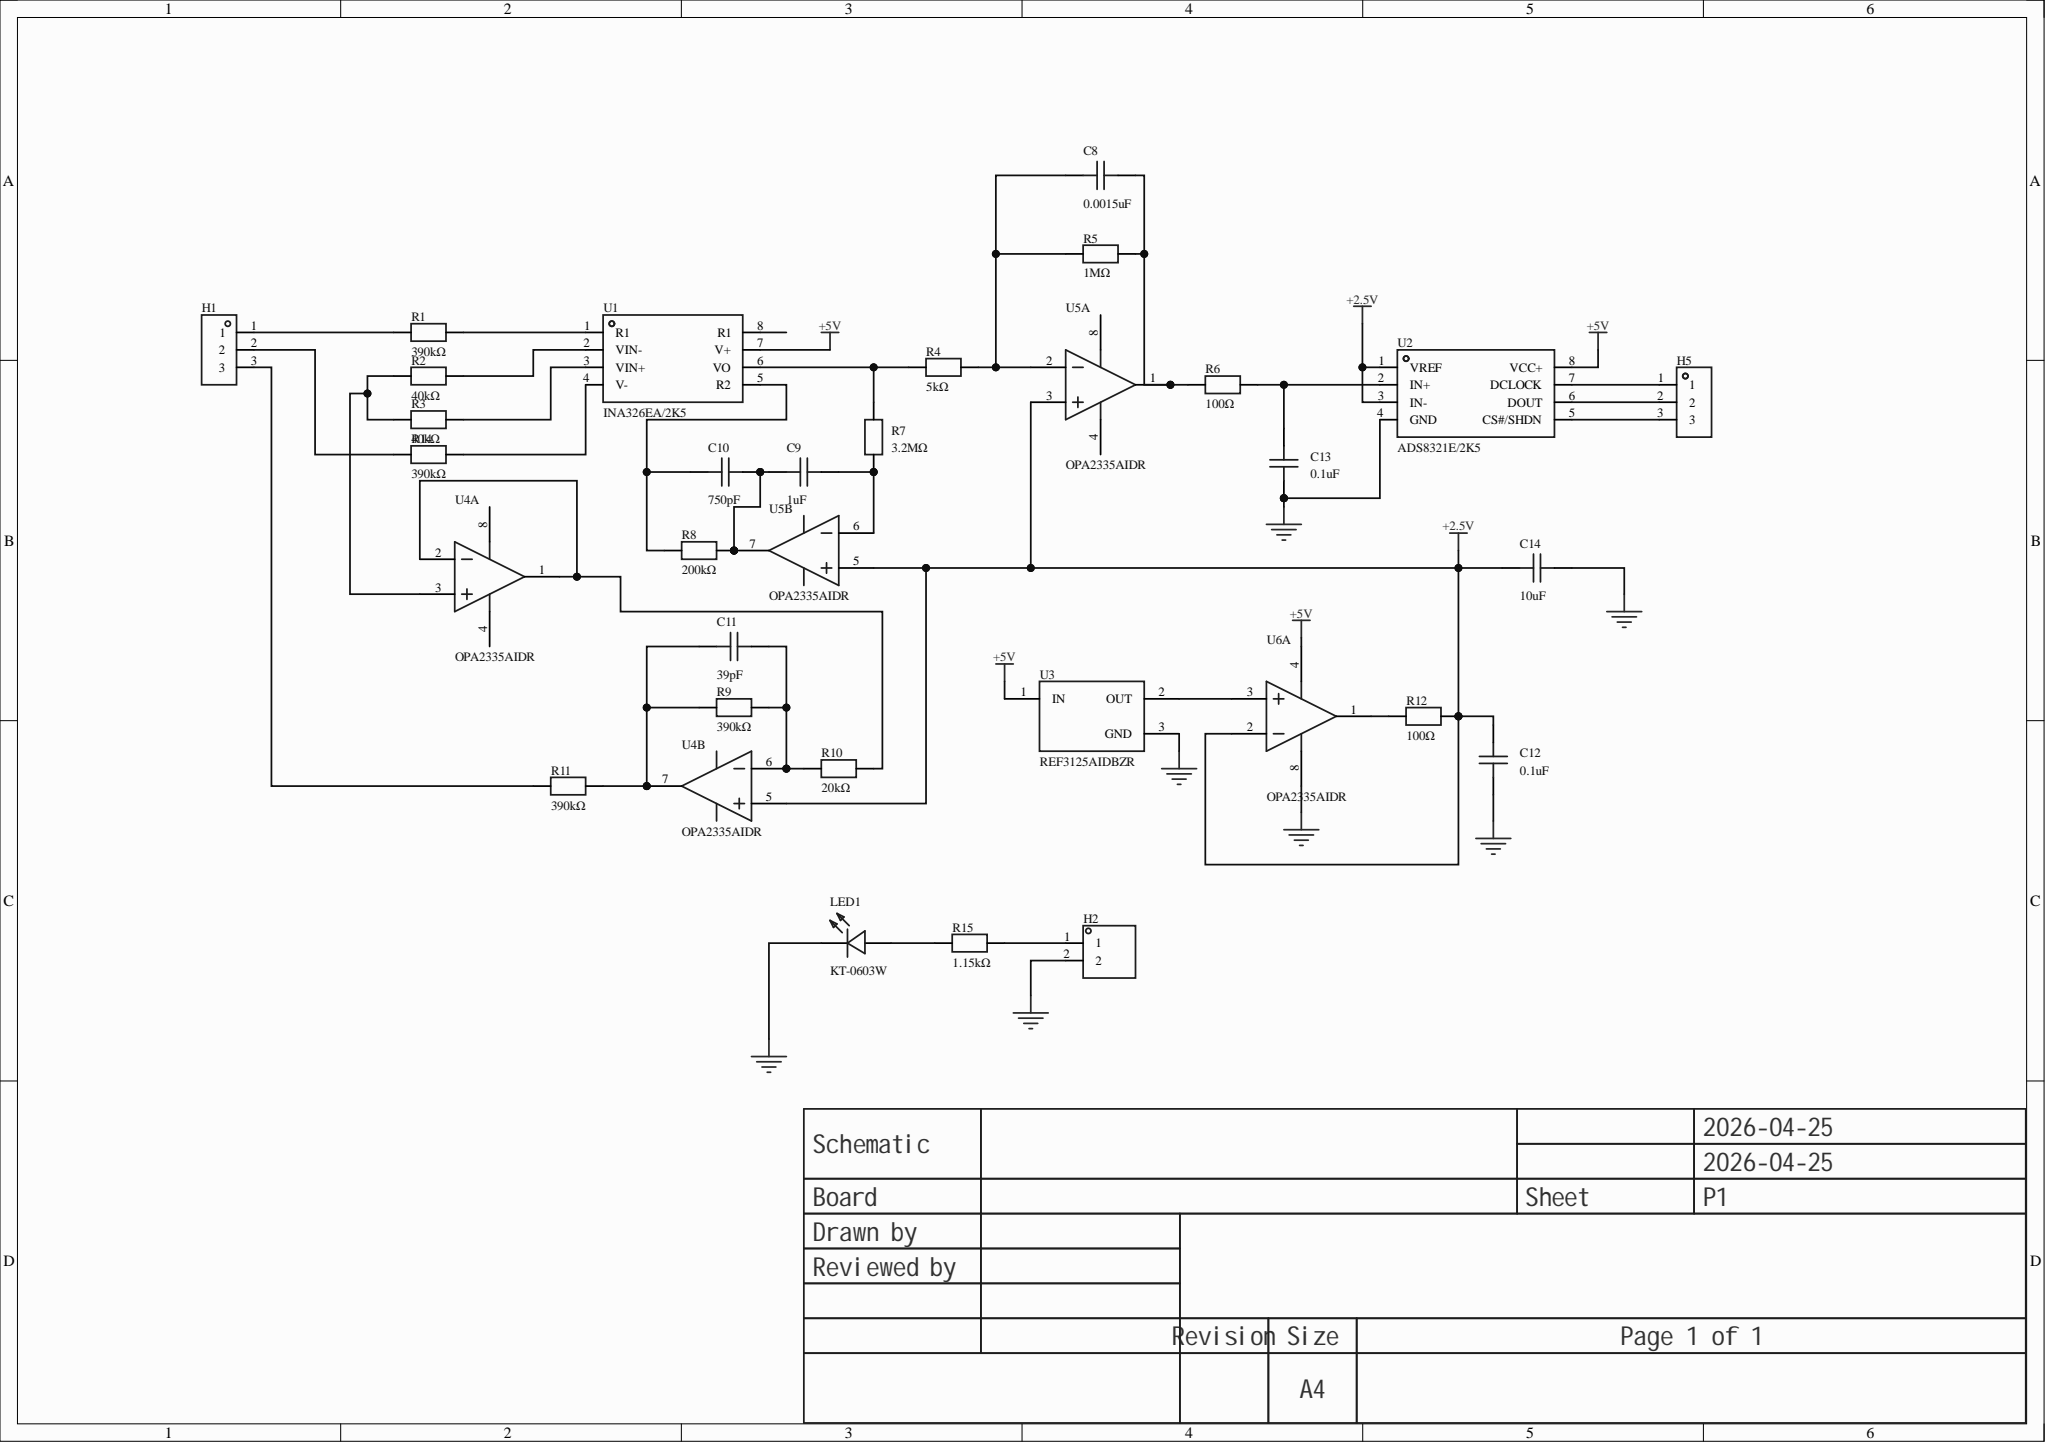Circuit board | Altium Designer | 31 parts | 28 nets
Bill of materials:
Comment,Description,Designator,Footprint,LibRef,Quantity
"0.0015uF","Capacitance: 22uF; Tolerance: ±20%; Rated voltage: 2.5V; Temperature coefficient: X7T;","C8","C0402","GRM158D70E226ME15D","1"
"1uF","Capacitance: 22uF; Tolerance: ±20%; Rated voltage: 2.5V; Temperature coefficient: X7T;","C9","C0402","GRM158D70E226ME15D","1"
"750pF","Capacitance: 22uF; Tolerance: ±20%; Rated voltage: 2.5V; Temperature coefficient: X7T;","C10","C0402","GRM158D70E226ME15D","1"
"39pF","Capacitance: 22uF; Tolerance: ±20%; Rated voltage: 2.5V; Temperature coefficient: X7T;","C11","C0402","GRM158D70E226ME15D","1"
"0.1uF","Capacitance: 22uF; Tolerance: ±20%; Rated voltage: 2.5V; Temperature coefficient: X7T;","C12, C13","C0402","GRM158D70E226ME15D","2"
"10uF","Capacitance: 22uF; Tolerance: ±20%; Rated voltage: 2.5V; Temperature coefficient: X7T;","C14","C0402","GRM158D70E226ME15D","1"
"","","H1, H5","HDR-TH_3P-P2.54-V-M","HDR-M_2.54_1x3P","2"
"","","H2","HDR-TH_2P-P2.54-V-M-1","HDR-M_2.54_1x2P","1"
"KT-0603W","","LED1","LED0603-R-RD_WHITE","KT-0603W","1"
"390kΩ","Resistor type: sampling resistor; alloy resistor; Resistance: 0Ω; Tolerance: ±1%; Power: 1W; Mounting: SMD;","R1, R9, R11","R1206","RE1206F1R000","3"
"40kΩ","Resistor type: sampling resistor; alloy resistor; Resistance: 0Ω; Tolerance: ±1%; Power: 1W; Mounting: SMD;","R2, R3","R1206","RE1206F1R000","2"
"5kΩ","Resistor type: sampling resistor; alloy resistor; Resistance: 0Ω; Tolerance: ±1%; Power: 1W; Mounting: SMD;","R4","R1206","RE1206F1R000","1"
"1MΩ","Resistor type: sampling resistor; alloy resistor; Resistance: 0Ω; Tolerance: ±1%; Power: 1W; Mounting: SMD;","R5","R1206","RE1206F1R000","1"
"100Ω","Resistor type: sampling resistor; alloy resistor; Resistance: 0Ω; Tolerance: ±1%; Power: 1W; Mounting: SMD;","R6, R12","R1206","RE1206F1R000","2"
"3.2MΩ","Resistor type: sampling resistor; alloy resistor; Resistance: 0Ω; Tolerance: ±1%; Power: 1W; Mounting: SMD;","R7","R1206","RE1206F1R000","1"
"200kΩ","Resistor type: sampling resistor; alloy resistor; Resistance: 0Ω; Tolerance: ±1%; Power: 1W; Mounting: SMD;","R8","R1206","RE1206F1R000","1"
"20kΩ","Resistor type: sampling resistor; alloy resistor; Resistance: 0Ω; Tolerance: ±1%; Power: 1W; Mounting: SMD;","R10","R1206","RE1206F1R000","1"
"390kΩ","Resistor type: thick film resistor; Resistance: 1.15kΩ; Tolerance: ±1%; Power: 62.5mW; Operating voltage: 50V;","R14","R0402","GR0402F1K15TAG00","1"
"1.15kΩ","Resistor type: thick film resistor; Resistance: 1.15kΩ; Tolerance: ±1%; Power: 62.5mW; Operating voltage: 50V;","R15","R0402","GR0402F1K15TAG00","1"
"INA326EA/2K5","","U1","VSSOP-8_L3.0-W3.0-P0.65-LS5.0-BL","INA326EA/2K5","1"
"ADS8321E/2K5","Resolution (bit): 16; Sample rate: 100kHz; Operating voltage: 4.75V~5.25V; Interface type: SPI;","U2","MSOP-8_L3.0-W3.0-P0.65-LS4.9-BL","ADS8321E/2K5","1"
"REF3125AIDBZR","Output type: Fixed; Operating voltage: 2.55V~5.5V; Output voltage: 2.5V; Output current: 10mA; Accuracy: ±0.2%;","U3","SOT-23-3_L2.9-W1.6-P1.90-LS2.8-BR","REF3125AIDBZR","1"
"OPA2335AIDR","Amplifier count: Dual; Gain bandwidth product (GBP): 2MHz; Input bias current (Ib): 70pA; Input offset voltage (Vos): 1uV; Slew rate (SR): 1.6V/us; Bandwidth (-3dB): -; Rail-to-rail: -;","U4, U5, U6","SOIC-8_L5.0-W4.0-P1.27-LS6.0-BL","OPA2335AIDR","3"
Netlist (Protel format):
[
C8
C0402
0.0015uF



]
[
C9
C0402
1uF



]
[
C10
C0402
750pF



]
[
C11
C0402
39pF



]
[
C12
C0402
0.1uF



]
[
C13
C0402
0.1uF



]
[
C14
C0402
10uF



]
[
H1
HDR-TH_3P-P2.54-V-M




]
[
H2
HDR-TH_2P-P2.54-V-M-1




]
[
H5
HDR-TH_3P-P2.54-V-M




]
[
LED1
LED0603-R-RD_WHITE
KT-0603W



]
[
R1
R1206
390kΩ



]
[
R2
R1206
40kΩ



]
[
R3
R1206
40kΩ



]
[
R4
R1206
5kΩ



]
[
R5
R1206
1MΩ



]
[
R6
R1206
100Ω



]
[
R7
R1206
3.2MΩ



]
[
R8
R1206
200kΩ



]
[
R9
R1206
390kΩ



]
[
R10
R1206
20kΩ



]
[
R11
R1206
390kΩ



]
[
R12
R1206
100Ω



]
[
R14
R0402
390kΩ



]
[
R15
R0402
1.15kΩ



]
[
U1
VSSOP-8_L3.0-W3.0-P0.65-LS5.0-BL
INA326EA/2K5



]
[
U2
MSOP-8_L3.0-W3.0-P0.65-LS4.9-BL
ADS8321E/2K5



]
[
U3
SOT-23-3_L2.9-W1.6-P1.90-LS2.8-BR
REF3125AIDBZR



]
[
U4
SOIC-8_L5.0-W4.0-P1.27-LS6.0-BL
OPA2335AIDR



]
[
U5
SOIC-8_L5.0-W4.0-P1.27-LS6.0-BL
OPA2335AIDR



]
[
U6
SOIC-8_L5.0-W4.0-P1.27-LS6.0-BL
OPA2335AIDR



]
(
NetU3_2
U3-2
U6-3
)
(
NetR14_2
R14-2
U1-4
)
(
NetR12_1
R12-1
U6-1
)
(
NetR10_2
R10-2
U4-1
U4-2
)
(
NetR4_1
R4-1
R7-2
U1-6
)
(
NetR3_2
R3-2
U1-3
)
(
NetR2_2
R2-2
U1-2
)
(
NetR2_1
R2-1
R3-1
U4-3
)
(
NetR1_2
R1-2
U1-1
)
(
NetLED1_1
LED1-1
R15-1
)
(
NetH5_3
H5-3
U2-5
)
(
NetH5_2
H5-2
U2-6
)
(
NetH5_1
H5-1
U2-7
)
(
NetH2_1
H2-1
R15-2
)
(
NetH1_3
H1-3
R11-1
)
(
NetH1_2
H1-2
R14-1
)
(
NetH1_1
H1-1
R1-1
)
(
NetC13_2
C13-2
R6-2
U2-2
)
(
NetC11_2
C11-2
R9-2
R10-1
U4-6
)
(
NetC11_1
C11-1
R9-1
R11-2
U4-7
)
(
NetC10_1
C10-1
R8-1
U1-5
)
(
NetC9_2
C9-2
R7-1
U5-6
)
(
NetC9_1
C9-1
C10-2
R8-2
U5-7
)
(
NetC8_2
C8-2
R5-2
R6-1
U5-1
)
(
NetC8_1
C8-1
R4-2
R5-1
U5-2
)
(
GND
C12-1
C13-1
C14-2
H2-2
LED1-2
U2-4
U3-3
U6-8
)
(
+5V
U1-7
U2-8
U3-1
U6-4
)
(
+2.5V
C12-2
C14-1
R12-2
U2-1
U2-3
U4-5
U5-3
U5-5
U6-2
)